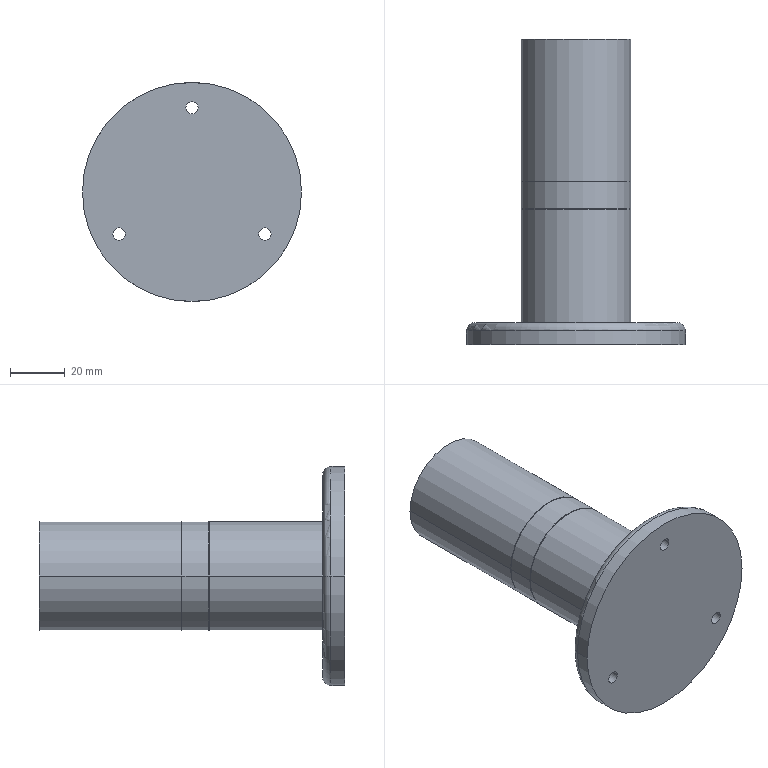Part | NX | 1 solid | 49 faces | box 80 x 111.49 x 80 mm | volume 113114 mm3 | cylinder 28 | plane 10 | torus 6 | cone 4 | sphere 1 | commonest cylinder face diameters 4.5 x6 6.5 x6 40 x6 10 x2 12 x2 36 x2
STEP:
#1=CARTESIAN_POINT('',(20.,-185.9,0.));
#2=VERTEX_POINT('',#1);
#3=CARTESIAN_POINT('',(-20.,-185.9,0.));
#4=VERTEX_POINT('',#3);
#5=CARTESIAN_POINT('',(0.,-185.9,0.));
#6=DIRECTION('',(0.,1.,0.));
#7=DIRECTION('',(1.,0.,0.));
#8=AXIS2_PLACEMENT_3D('',#5,#6,#7);
#9=CIRCLE('',#8,20.);
#10=EDGE_CURVE('',#2,#4,#9,.T.);
#11=ORIENTED_EDGE('',*,*,#10,.F.);
#12=CARTESIAN_POINT('',(19.9,-186.,0.));
#13=VERTEX_POINT('',#12);
#14=CARTESIAN_POINT('',(19.9,-185.9,0.));
#15=DIRECTION('',(0.,0.,1.));
#16=DIRECTION('',(1.,0.,0.));
#17=AXIS2_PLACEMENT_3D('',#14,#15,#16);
#18=CIRCLE('',#17,0.1);
#19=EDGE_CURVE('',#13,#2,#18,.T.);
#20=ORIENTED_EDGE('',*,*,#19,.F.);
#21=CARTESIAN_POINT('',(-19.9,-186.,0.));
#22=VERTEX_POINT('',#21);
#23=CARTESIAN_POINT('',(0.,-186.,0.));
#24=DIRECTION('',(0.,1.,0.));
#25=DIRECTION('',(-1.,0.,0.));
#26=AXIS2_PLACEMENT_3D('',#23,#24,#25);
#27=CIRCLE('',#26,19.9);
#28=EDGE_CURVE('',#13,#22,#27,.T.);
#29=ORIENTED_EDGE('',*,*,#28,.T.);
#30=CARTESIAN_POINT('',(-19.9,-185.9,0.));
#31=DIRECTION('',(0.,0.,-1.));
#32=DIRECTION('',(-1.,0.,0.));
#33=AXIS2_PLACEMENT_3D('',#30,#31,#32);
#34=CIRCLE('',#33,0.1);
#35=EDGE_CURVE('',#22,#4,#34,.T.);
#36=ORIENTED_EDGE('',*,*,#35,.T.);
#37=EDGE_LOOP('',(#11,#20,#29,#36));
#38=FACE_BOUND('',#37,.T.);
#39=CARTESIAN_POINT('',(0.,-185.9,0.));
#40=DIRECTION('',(0.,-1.,0.));
#41=DIRECTION('',(-1.,0.,0.));
#42=AXIS2_PLACEMENT_3D('',#39,#40,#41);
#43=TOROIDAL_SURFACE('',#42,19.9,0.1);
#44=ADVANCED_FACE('',(#38),#43,.T.);
#45=CARTESIAN_POINT('',(-40.,-230.5,0.));
#46=VERTEX_POINT('',#45);
#47=CARTESIAN_POINT('',(-37.,-227.5,0.));
#48=VERTEX_POINT('',#47);
#49=CARTESIAN_POINT('',(-37.,-230.5,0.));
#50=DIRECTION('',(0.,0.,-1.));
#51=DIRECTION('',(-1.,0.,0.));
#52=AXIS2_PLACEMENT_3D('',#49,#50,#51);
#53=CIRCLE('',#52,3.);
#54=EDGE_CURVE('',#46,#48,#53,.T.);
#55=ORIENTED_EDGE('',*,*,#54,.T.);
#56=CARTESIAN_POINT('',(37.,-227.5,0.));
#57=VERTEX_POINT('',#56);
#58=CARTESIAN_POINT('',(0.,-227.5,0.));
#59=DIRECTION('',(0.,-1.,0.));
#60=DIRECTION('',(1.,0.,0.));
#61=AXIS2_PLACEMENT_3D('',#58,#59,#60);
#62=CIRCLE('',#61,37.);
#63=EDGE_CURVE('',#48,#57,#62,.T.);
#64=ORIENTED_EDGE('',*,*,#63,.T.);
#65=CARTESIAN_POINT('',(40.,-230.5,0.));
#66=VERTEX_POINT('',#65);
#67=CARTESIAN_POINT('',(37.,-230.5,0.));
#68=DIRECTION('',(0.,0.,1.));
#69=DIRECTION('',(1.,0.,0.));
#70=AXIS2_PLACEMENT_3D('',#67,#68,#69);
#71=CIRCLE('',#70,3.);
#72=EDGE_CURVE('',#66,#57,#71,.T.);
#73=ORIENTED_EDGE('',*,*,#72,.F.);
#74=CARTESIAN_POINT('',(0.,-230.5,0.));
#75=DIRECTION('',(0.,-1.,0.));
#76=DIRECTION('',(-1.,0.,0.));
#77=AXIS2_PLACEMENT_3D('',#74,#75,#76);
#78=CIRCLE('',#77,40.);
#79=EDGE_CURVE('',#46,#66,#78,.T.);
#80=ORIENTED_EDGE('',*,*,#79,.F.);
#81=EDGE_LOOP('',(#55,#64,#73,#80));
#82=FACE_BOUND('',#81,.T.);
#83=CARTESIAN_POINT('',(0.,-230.5,0.));
#84=DIRECTION('',(0.,-1.,0.));
#85=DIRECTION('',(-1.,0.,0.));
#86=AXIS2_PLACEMENT_3D('',#83,#84,#85);
#87=TOROIDAL_SURFACE('',#86,37.,3.);
#88=ADVANCED_FACE('',(#82),#87,.T.);
#89=CARTESIAN_POINT('',(-20.,-186.1,0.));
#90=VERTEX_POINT('',#89);
#91=CARTESIAN_POINT('',(-19.9,-186.1,0.));
#92=DIRECTION('',(0.,0.,-1.));
#93=DIRECTION('',(-1.,0.,0.));
#94=AXIS2_PLACEMENT_3D('',#91,#92,#93);
#95=CIRCLE('',#94,0.1);
#96=EDGE_CURVE('',#90,#22,#95,.T.);
#97=ORIENTED_EDGE('',*,*,#96,.T.);
#98=ORIENTED_EDGE('',*,*,#28,.F.);
#99=CARTESIAN_POINT('',(20.,-186.1,0.));
#100=VERTEX_POINT('',#99);
#101=CARTESIAN_POINT('',(19.9,-186.1,0.));
#102=DIRECTION('',(0.,0.,1.));
#103=DIRECTION('',(1.,0.,0.));
#104=AXIS2_PLACEMENT_3D('',#101,#102,#103);
#105=CIRCLE('',#104,0.1);
#106=EDGE_CURVE('',#100,#13,#105,.T.);
#107=ORIENTED_EDGE('',*,*,#106,.F.);
#108=CARTESIAN_POINT('',(0.,-186.1,0.));
#109=DIRECTION('',(0.,-1.,0.));
#110=DIRECTION('',(-1.,0.,0.));
#111=AXIS2_PLACEMENT_3D('',#108,#109,#110);
#112=CIRCLE('',#111,20.);
#113=EDGE_CURVE('',#90,#100,#112,.T.);
#114=ORIENTED_EDGE('',*,*,#113,.F.);
#115=EDGE_LOOP('',(#97,#98,#107,#114));
#116=FACE_BOUND('',#115,.T.);
#117=CARTESIAN_POINT('',(0.,-186.1,0.));
#118=DIRECTION('',(0.,-1.,0.));
#119=DIRECTION('',(-1.,0.,0.));
#120=AXIS2_PLACEMENT_3D('',#117,#118,#119);
#121=TOROIDAL_SURFACE('',#120,19.9,0.1);
#122=ADVANCED_FACE('',(#116),#121,.T.);
#123=CARTESIAN_POINT('',(-18.,-175.95,0.));
#124=VERTEX_POINT('',#123);
#125=CARTESIAN_POINT('',(-18.,-124.01,0.));
#126=VERTEX_POINT('',#125);
#127=CARTESIAN_POINT('',(-18.,-120.91,0.));
#128=DIRECTION('',(0.,-1.,0.));
#129=VECTOR('',#128,1000.);
#130=LINE('',#127,#129);
#131=EDGE_CURVE('',#124,#126,#130,.F.);
#132=ORIENTED_EDGE('',*,*,#131,.T.);
#133=CARTESIAN_POINT('',(18.,-124.01,0.));
#134=VERTEX_POINT('',#133);
#135=CARTESIAN_POINT('',(0.,-124.01,0.));
#136=DIRECTION('',(0.,1.,0.));
#137=DIRECTION('',(1.,0.,0.));
#138=AXIS2_PLACEMENT_3D('',#135,#136,#137);
#139=CIRCLE('',#138,18.);
#140=EDGE_CURVE('',#126,#134,#139,.T.);
#141=ORIENTED_EDGE('',*,*,#140,.T.);
#142=CARTESIAN_POINT('',(18.,-175.95,0.));
#143=VERTEX_POINT('',#142);
#144=CARTESIAN_POINT('',(18.,-120.91,0.));
#145=DIRECTION('',(0.,-1.,0.));
#146=VECTOR('',#145,1000.);
#147=LINE('',#144,#146);
#148=EDGE_CURVE('',#143,#134,#147,.F.);
#149=ORIENTED_EDGE('',*,*,#148,.F.);
#150=CARTESIAN_POINT('',(0.,-175.95,0.));
#151=DIRECTION('',(0.,-1.,0.));
#152=DIRECTION('',(1.,0.,0.));
#153=AXIS2_PLACEMENT_3D('',#150,#151,#152);
#154=CIRCLE('',#153,18.);
#155=EDGE_CURVE('',#143,#124,#154,.T.);
#156=ORIENTED_EDGE('',*,*,#155,.T.);
#157=EDGE_LOOP('',(#132,#141,#149,#156));
#158=FACE_BOUND('',#157,.T.);
#159=CARTESIAN_POINT('',(0.,-120.91,0.));
#160=DIRECTION('',(0.,-1.,0.));
#161=DIRECTION('',(-1.,0.,0.));
#162=AXIS2_PLACEMENT_3D('',#159,#160,#161);
#163=CYLINDRICAL_SURFACE('',#162,18.);
#164=ADVANCED_FACE('',(#158),#163,.F.);
#165=CARTESIAN_POINT('',(-2.25,-229.5,30.75));
#166=VERTEX_POINT('',#165);
#167=CARTESIAN_POINT('',(2.25,-229.5,30.75));
#168=VERTEX_POINT('',#167);
#169=CARTESIAN_POINT('',(0.,-229.5,30.75));
#170=DIRECTION('',(0.,1.,0.));
#171=DIRECTION('',(1.,0.,0.));
#172=AXIS2_PLACEMENT_3D('',#169,#170,#171);
#173=CIRCLE('',#172,2.25);
#174=EDGE_CURVE('',#166,#168,#173,.T.);
#175=ORIENTED_EDGE('',*,*,#174,.T.);
#176=CARTESIAN_POINT('',(2.25,-235.5,30.75));
#177=VERTEX_POINT('',#176);
#178=CARTESIAN_POINT('',(2.25,-511.752,30.75));
#179=DIRECTION('',(0.,1.,0.));
#180=VECTOR('',#179,1000.);
#181=LINE('',#178,#180);
#182=EDGE_CURVE('',#177,#168,#181,.T.);
#183=ORIENTED_EDGE('',*,*,#182,.F.);
#184=CARTESIAN_POINT('',(-2.25,-235.5,30.75));
#185=VERTEX_POINT('',#184);
#186=CARTESIAN_POINT('',(0.,-235.5,30.75));
#187=DIRECTION('',(0.,-1.,0.));
#188=DIRECTION('',(1.,0.,0.));
#189=AXIS2_PLACEMENT_3D('',#186,#187,#188);
#190=CIRCLE('',#189,2.25);
#191=EDGE_CURVE('',#177,#185,#190,.T.);
#192=ORIENTED_EDGE('',*,*,#191,.T.);
#193=CARTESIAN_POINT('',(-2.25,-511.752,30.75));
#194=DIRECTION('',(0.,1.,0.));
#195=VECTOR('',#194,1000.);
#196=LINE('',#193,#195);
#197=EDGE_CURVE('',#185,#166,#196,.T.);
#198=ORIENTED_EDGE('',*,*,#197,.T.);
#199=EDGE_LOOP('',(#175,#183,#192,#198));
#200=FACE_BOUND('',#199,.T.);
#201=CARTESIAN_POINT('',(0.,-511.752,30.75));
#202=DIRECTION('',(0.,1.,0.));
#203=DIRECTION('',(1.,0.,0.));
#204=AXIS2_PLACEMENT_3D('',#201,#202,#203);
#205=CYLINDRICAL_SURFACE('',#204,2.25);
#206=ADVANCED_FACE('',(#200),#205,.F.);
#207=CARTESIAN_POINT('',(29.88,-227.5,-15.375));
#208=VERTEX_POINT('',#207);
#209=CARTESIAN_POINT('',(29.88,-229.5,-15.375));
#210=VERTEX_POINT('',#209);
#211=CARTESIAN_POINT('',(29.88,-503.23,-15.375));
#212=DIRECTION('',(0.,1.,0.));
#213=VECTOR('',#212,1000.);
#214=LINE('',#211,#213);
#215=EDGE_CURVE('',#208,#210,#214,.F.);
#216=ORIENTED_EDGE('',*,*,#215,.F.);
#217=CARTESIAN_POINT('',(23.38,-227.5,-15.375));
#218=VERTEX_POINT('',#217);
#219=CARTESIAN_POINT('',(26.63,-227.5,-15.375));
#220=DIRECTION('',(0.,1.,0.));
#221=DIRECTION('',(-1.,0.,0.));
#222=AXIS2_PLACEMENT_3D('',#219,#220,#221);
#223=CIRCLE('',#222,3.25);
#224=EDGE_CURVE('',#208,#218,#223,.T.);
#225=ORIENTED_EDGE('',*,*,#224,.T.);
#226=CARTESIAN_POINT('',(23.38,-229.5,-15.375));
#227=VERTEX_POINT('',#226);
#228=CARTESIAN_POINT('',(23.38,-503.23,-15.375));
#229=DIRECTION('',(0.,1.,0.));
#230=VECTOR('',#229,1000.);
#231=LINE('',#228,#230);
#232=EDGE_CURVE('',#218,#227,#231,.F.);
#233=ORIENTED_EDGE('',*,*,#232,.T.);
#234=CARTESIAN_POINT('',(26.63,-229.5,-15.375));
#235=DIRECTION('',(0.,-1.,0.));
#236=DIRECTION('',(1.,0.,0.));
#237=AXIS2_PLACEMENT_3D('',#234,#235,#236);
#238=CIRCLE('',#237,3.25);
#239=EDGE_CURVE('',#227,#210,#238,.T.);
#240=ORIENTED_EDGE('',*,*,#239,.T.);
#241=EDGE_LOOP('',(#216,#225,#233,#240));
#242=FACE_BOUND('',#241,.T.);
#243=CARTESIAN_POINT('',(26.63,-503.23,-15.375));
#244=DIRECTION('',(0.,1.,0.));
#245=DIRECTION('',(1.,0.,0.));
#246=AXIS2_PLACEMENT_3D('',#243,#244,#245);
#247=CYLINDRICAL_SURFACE('',#246,3.25);
#248=ADVANCED_FACE('',(#242),#247,.F.);
#249=CARTESIAN_POINT('',(-23.38,-227.5,-15.375));
#250=VERTEX_POINT('',#249);
#251=CARTESIAN_POINT('',(-23.38,-229.5,-15.375));
#252=VERTEX_POINT('',#251);
#253=CARTESIAN_POINT('',(-23.38,-503.23,-15.375));
#254=DIRECTION('',(0.,1.,0.));
#255=VECTOR('',#254,1000.);
#256=LINE('',#253,#255);
#257=EDGE_CURVE('',#250,#252,#256,.F.);
#258=ORIENTED_EDGE('',*,*,#257,.F.);
#259=CARTESIAN_POINT('',(-29.88,-227.5,-15.375));
#260=VERTEX_POINT('',#259);
#261=CARTESIAN_POINT('',(-26.63,-227.5,-15.375));
#262=DIRECTION('',(0.,1.,0.));
#263=DIRECTION('',(-1.,0.,0.));
#264=AXIS2_PLACEMENT_3D('',#261,#262,#263);
#265=CIRCLE('',#264,3.25);
#266=EDGE_CURVE('',#250,#260,#265,.T.);
#267=ORIENTED_EDGE('',*,*,#266,.T.);
#268=CARTESIAN_POINT('',(-29.88,-229.5,-15.375));
#269=VERTEX_POINT('',#268);
#270=CARTESIAN_POINT('',(-29.88,-503.23,-15.375));
#271=DIRECTION('',(0.,1.,0.));
#272=VECTOR('',#271,1000.);
#273=LINE('',#270,#272);
#274=EDGE_CURVE('',#260,#269,#273,.F.);
#275=ORIENTED_EDGE('',*,*,#274,.T.);
#276=CARTESIAN_POINT('',(-26.63,-229.5,-15.375));
#277=DIRECTION('',(0.,-1.,0.));
#278=DIRECTION('',(1.,0.,0.));
#279=AXIS2_PLACEMENT_3D('',#276,#277,#278);
#280=CIRCLE('',#279,3.25);
#281=EDGE_CURVE('',#269,#252,#280,.T.);
#282=ORIENTED_EDGE('',*,*,#281,.T.);
#283=EDGE_LOOP('',(#258,#267,#275,#282));
#284=FACE_BOUND('',#283,.T.);
#285=CARTESIAN_POINT('',(-26.63,-503.23,-15.375));
#286=DIRECTION('',(0.,1.,0.));
#287=DIRECTION('',(1.,0.,0.));
#288=AXIS2_PLACEMENT_3D('',#285,#286,#287);
#289=CYLINDRICAL_SURFACE('',#288,3.25);
#290=ADVANCED_FACE('',(#284),#289,.F.);
#291=CARTESIAN_POINT('',(-20.,-176.05,0.));
#292=VERTEX_POINT('',#291);
#293=CARTESIAN_POINT('',(-19.95,-176.,0.));
#294=VERTEX_POINT('',#293);
#295=CARTESIAN_POINT('',(-19.975,-176.025,0.));
#296=DIRECTION('',(-0.7071,-0.7071,0.));
#297=VECTOR('',#296,1000.);
#298=LINE('',#295,#297);
#299=EDGE_CURVE('',#292,#294,#298,.F.);
#300=ORIENTED_EDGE('',*,*,#299,.F.);
#301=CARTESIAN_POINT('',(20.,-176.05,0.));
#302=VERTEX_POINT('',#301);
#303=CARTESIAN_POINT('',(0.,-176.05,0.));
#304=DIRECTION('',(0.,-1.,0.));
#305=DIRECTION('',(1.,0.,0.));
#306=AXIS2_PLACEMENT_3D('',#303,#304,#305);
#307=CIRCLE('',#306,20.);
#308=EDGE_CURVE('',#302,#292,#307,.T.);
#309=ORIENTED_EDGE('',*,*,#308,.F.);
#310=CARTESIAN_POINT('',(19.95,-176.,0.));
#311=VERTEX_POINT('',#310);
#312=CARTESIAN_POINT('',(19.975,-176.025,0.));
#313=DIRECTION('',(0.7071,-0.7071,0.));
#314=VECTOR('',#313,1000.);
#315=LINE('',#312,#314);
#316=EDGE_CURVE('',#302,#311,#315,.F.);
#317=ORIENTED_EDGE('',*,*,#316,.T.);
#318=CARTESIAN_POINT('',(0.,-176.,0.));
#319=DIRECTION('',(0.,1.,0.));
#320=DIRECTION('',(-1.,0.,0.));
#321=AXIS2_PLACEMENT_3D('',#318,#319,#320);
#322=CIRCLE('',#321,19.95);
#323=EDGE_CURVE('',#294,#311,#322,.T.);
#324=ORIENTED_EDGE('',*,*,#323,.F.);
#325=EDGE_LOOP('',(#300,#309,#317,#324));
#326=FACE_BOUND('',#325,.T.);
#327=CARTESIAN_POINT('',(0.,-176.025,0.));
#328=DIRECTION('',(0.,-1.,0.));
#329=DIRECTION('',(-1.,0.,0.));
#330=AXIS2_PLACEMENT_3D('',#327,#328,#329);
#331=CONICAL_SURFACE('',#330,19.975,0.7854);
#332=ADVANCED_FACE('',(#326),#331,.T.);
#333=CARTESIAN_POINT('',(-19.85,-175.95,0.));
#334=VERTEX_POINT('',#333);
#335=CARTESIAN_POINT('',(-19.85,-176.,0.));
#336=VERTEX_POINT('',#335);
#337=CARTESIAN_POINT('',(-19.85,-120.91,0.));
#338=DIRECTION('',(0.,-1.,0.));
#339=VECTOR('',#338,1000.);
#340=LINE('',#337,#339);
#341=EDGE_CURVE('',#334,#336,#340,.T.);
#342=ORIENTED_EDGE('',*,*,#341,.F.);
#343=CARTESIAN_POINT('',(19.85,-175.95,0.));
#344=VERTEX_POINT('',#343);
#345=CARTESIAN_POINT('',(0.,-175.95,0.));
#346=DIRECTION('',(0.,1.,0.));
#347=DIRECTION('',(1.,0.,0.));
#348=AXIS2_PLACEMENT_3D('',#345,#346,#347);
#349=CIRCLE('',#348,19.85);
#350=EDGE_CURVE('',#334,#344,#349,.T.);
#351=ORIENTED_EDGE('',*,*,#350,.T.);
#352=CARTESIAN_POINT('',(19.85,-176.,0.));
#353=VERTEX_POINT('',#352);
#354=CARTESIAN_POINT('',(19.85,-120.91,0.));
#355=DIRECTION('',(0.,-1.,0.));
#356=VECTOR('',#355,1000.);
#357=LINE('',#354,#356);
#358=EDGE_CURVE('',#344,#353,#357,.T.);
#359=ORIENTED_EDGE('',*,*,#358,.T.);
#360=CARTESIAN_POINT('',(0.,-176.,0.));
#361=DIRECTION('',(0.,-1.,0.));
#362=DIRECTION('',(1.,0.,0.));
#363=AXIS2_PLACEMENT_3D('',#360,#361,#362);
#364=CIRCLE('',#363,19.85);
#365=EDGE_CURVE('',#353,#336,#364,.T.);
#366=ORIENTED_EDGE('',*,*,#365,.T.);
#367=EDGE_LOOP('',(#342,#351,#359,#366));
#368=FACE_BOUND('',#367,.T.);
#369=CARTESIAN_POINT('',(0.,-120.91,0.));
#370=DIRECTION('',(0.,-1.,0.));
#371=DIRECTION('',(-1.,0.,0.));
#372=AXIS2_PLACEMENT_3D('',#369,#370,#371);
#373=CYLINDRICAL_SURFACE('',#372,19.85);
#374=ADVANCED_FACE('',(#368),#373,.F.);
#375=CARTESIAN_POINT('',(-40.,-235.5,0.));
#376=VERTEX_POINT('',#375);
#377=CARTESIAN_POINT('',(-40.,-227.1,0.));
#378=DIRECTION('',(0.,-1.,0.));
#379=VECTOR('',#378,1000.);
#380=LINE('',#377,#379);
#381=EDGE_CURVE('',#376,#46,#380,.F.);
#382=ORIENTED_EDGE('',*,*,#381,.T.);
#383=ORIENTED_EDGE('',*,*,#79,.T.);
#384=CARTESIAN_POINT('',(40.,-235.5,0.));
#385=VERTEX_POINT('',#384);
#386=CARTESIAN_POINT('',(40.,-227.1,0.));
#387=DIRECTION('',(0.,-1.,0.));
#388=VECTOR('',#387,1000.);
#389=LINE('',#386,#388);
#390=EDGE_CURVE('',#385,#66,#389,.F.);
#391=ORIENTED_EDGE('',*,*,#390,.F.);
#392=CARTESIAN_POINT('',(0.,-235.5,0.));
#393=DIRECTION('',(0.,1.,0.));
#394=DIRECTION('',(1.,0.,0.));
#395=AXIS2_PLACEMENT_3D('',#392,#393,#394);
#396=CIRCLE('',#395,40.);
#397=EDGE_CURVE('',#385,#376,#396,.T.);
#398=ORIENTED_EDGE('',*,*,#397,.T.);
#399=EDGE_LOOP('',(#382,#383,#391,#398));
#400=FACE_BOUND('',#399,.T.);
#401=CARTESIAN_POINT('',(0.,-227.1,0.));
#402=DIRECTION('',(0.,-1.,0.));
#403=DIRECTION('',(-1.,0.,0.));
#404=AXIS2_PLACEMENT_3D('',#401,#402,#403);
#405=CYLINDRICAL_SURFACE('',#404,40.);
#406=ADVANCED_FACE('',(#400),#405,.T.);
#407=CARTESIAN_POINT('',(24.38,-229.5,-15.375));
#408=VERTEX_POINT('',#407);
#409=CARTESIAN_POINT('',(28.88,-229.5,-15.375));
#410=VERTEX_POINT('',#409);
#411=CARTESIAN_POINT('',(26.63,-229.5,-15.375));
#412=DIRECTION('',(0.,1.,0.));
#413=DIRECTION('',(1.,0.,0.));
#414=AXIS2_PLACEMENT_3D('',#411,#412,#413);
#415=CIRCLE('',#414,2.25);
#416=EDGE_CURVE('',#408,#410,#415,.T.);
#417=ORIENTED_EDGE('',*,*,#416,.T.);
#418=CARTESIAN_POINT('',(28.88,-235.5,-15.375));
#419=VERTEX_POINT('',#418);
#420=CARTESIAN_POINT('',(28.88,-503.23,-15.375));
#421=DIRECTION('',(0.,1.,0.));
#422=VECTOR('',#421,1000.);
#423=LINE('',#420,#422);
#424=EDGE_CURVE('',#419,#410,#423,.T.);
#425=ORIENTED_EDGE('',*,*,#424,.F.);
#426=CARTESIAN_POINT('',(24.38,-235.5,-15.375));
#427=VERTEX_POINT('',#426);
#428=CARTESIAN_POINT('',(26.63,-235.5,-15.375));
#429=DIRECTION('',(0.,-1.,0.));
#430=DIRECTION('',(1.,0.,0.));
#431=AXIS2_PLACEMENT_3D('',#428,#429,#430);
#432=CIRCLE('',#431,2.25);
#433=EDGE_CURVE('',#419,#427,#432,.T.);
#434=ORIENTED_EDGE('',*,*,#433,.T.);
#435=CARTESIAN_POINT('',(24.38,-503.23,-15.375));
#436=DIRECTION('',(0.,1.,0.));
#437=VECTOR('',#436,1000.);
#438=LINE('',#435,#437);
#439=EDGE_CURVE('',#427,#408,#438,.T.);
#440=ORIENTED_EDGE('',*,*,#439,.T.);
#441=EDGE_LOOP('',(#417,#425,#434,#440));
#442=FACE_BOUND('',#441,.T.);
#443=CARTESIAN_POINT('',(26.63,-503.23,-15.375));
#444=DIRECTION('',(0.,1.,0.));
#445=DIRECTION('',(1.,0.,0.));
#446=AXIS2_PLACEMENT_3D('',#443,#444,#445);
#447=CYLINDRICAL_SURFACE('',#446,2.25);
#448=ADVANCED_FACE('',(#442),#447,.F.);
#449=CARTESIAN_POINT('',(-24.38,-235.5,-15.375));
#450=VERTEX_POINT('',#449);
#451=CARTESIAN_POINT('',(-24.38,-229.5,-15.375));
#452=VERTEX_POINT('',#451);
#453=CARTESIAN_POINT('',(-24.38,-503.23,-15.375));
#454=DIRECTION('',(0.,1.,0.));
#455=VECTOR('',#454,1000.);
#456=LINE('',#453,#455);
#457=EDGE_CURVE('',#450,#452,#456,.T.);
#458=ORIENTED_EDGE('',*,*,#457,.F.);
#459=CARTESIAN_POINT('',(-28.88,-235.5,-15.375));
#460=VERTEX_POINT('',#459);
#461=CARTESIAN_POINT('',(-26.63,-235.5,-15.375));
#462=DIRECTION('',(0.,-1.,0.));
#463=DIRECTION('',(1.,0.,0.));
#464=AXIS2_PLACEMENT_3D('',#461,#462,#463);
#465=CIRCLE('',#464,2.25);
#466=EDGE_CURVE('',#450,#460,#465,.T.);
#467=ORIENTED_EDGE('',*,*,#466,.T.);
#468=CARTESIAN_POINT('',(-28.88,-229.5,-15.375));
#469=VERTEX_POINT('',#468);
#470=CARTESIAN_POINT('',(-28.88,-503.23,-15.375));
#471=DIRECTION('',(0.,1.,0.));
#472=VECTOR('',#471,1000.);
#473=LINE('',#470,#472);
#474=EDGE_CURVE('',#460,#469,#473,.T.);
#475=ORIENTED_EDGE('',*,*,#474,.T.);
#476=CARTESIAN_POINT('',(-26.63,-229.5,-15.375));
#477=DIRECTION('',(0.,1.,0.));
#478=DIRECTION('',(-1.,0.,0.));
#479=AXIS2_PLACEMENT_3D('',#476,#477,#478);
#480=CIRCLE('',#479,2.25);
#481=EDGE_CURVE('',#469,#452,#480,.T.);
#482=ORIENTED_EDGE('',*,*,#481,.T.);
#483=EDGE_LOOP('',(#458,#467,#475,#482));
#484=FACE_BOUND('',#483,.T.);
#485=CARTESIAN_POINT('',(-26.63,-503.23,-15.375));
#486=DIRECTION('',(0.,1.,0.));
#487=DIRECTION('',(1.,0.,0.));
#488=AXIS2_PLACEMENT_3D('',#485,#486,#487);
#489=CYLINDRICAL_SURFACE('',#488,2.25);
#490=ADVANCED_FACE('',(#484),#489,.F.);
#491=CARTESIAN_POINT('',(-20.,-227.5,0.));
#492=VERTEX_POINT('',#491);
#493=CARTESIAN_POINT('',(-20.,-183.925,0.));
#494=DIRECTION('',(0.,-1.,0.));
#495=VECTOR('',#494,1000.);
#496=LINE('',#493,#495);
#497=EDGE_CURVE('',#492,#90,#496,.F.);
#498=ORIENTED_EDGE('',*,*,#497,.T.);
#499=ORIENTED_EDGE('',*,*,#113,.T.);
#500=CARTESIAN_POINT('',(20.,-227.5,0.));
#501=VERTEX_POINT('',#500);
#502=CARTESIAN_POINT('',(20.,-183.925,0.));
#503=DIRECTION('',(0.,-1.,0.));
#504=VECTOR('',#503,1000.);
#505=LINE('',#502,#504);
#506=EDGE_CURVE('',#501,#100,#505,.F.);
#507=ORIENTED_EDGE('',*,*,#506,.F.);
#508=CARTESIAN_POINT('',(0.,-227.5,0.));
#509=DIRECTION('',(0.,1.,0.));
#510=DIRECTION('',(1.,0.,0.));
#511=AXIS2_PLACEMENT_3D('',#508,#509,#510);
#512=CIRCLE('',#511,20.);
#513=EDGE_CURVE('',#501,#492,#512,.T.);
#514=ORIENTED_EDGE('',*,*,#513,.T.);
#515=EDGE_LOOP('',(#498,#499,#507,#514));
#516=FACE_BOUND('',#515,.T.);
#517=CARTESIAN_POINT('',(0.,-183.925,0.));
#518=DIRECTION('',(0.,-1.,0.));
#519=DIRECTION('',(-1.,0.,0.));
#520=AXIS2_PLACEMENT_3D('',#517,#518,#519);
#521=CYLINDRICAL_SURFACE('',#520,20.);
#522=ADVANCED_FACE('',(#516),#521,.T.);
#523=CARTESIAN_POINT('',(-20.,-120.91,0.));
#524=DIRECTION('',(0.,-1.,0.));
#525=VECTOR('',#524,1000.);
#526=LINE('',#523,#525);
#527=EDGE_CURVE('',#4,#292,#526,.F.);
#528=ORIENTED_EDGE('',*,*,#527,.F.);
#529=CARTESIAN_POINT('',(0.,-185.9,0.));
#530=DIRECTION('',(0.,1.,0.));
#531=DIRECTION('',(1.,0.,0.));
#532=AXIS2_PLACEMENT_3D('',#529,#530,#531);
#533=CIRCLE('',#532,20.);
#534=EDGE_CURVE('',#4,#2,#533,.T.);
#535=ORIENTED_EDGE('',*,*,#534,.T.);
#536=CARTESIAN_POINT('',(20.,-120.91,0.));
#537=DIRECTION('',(0.,-1.,0.));
#538=VECTOR('',#537,1000.);
#539=LINE('',#536,#538);
#540=EDGE_CURVE('',#2,#302,#539,.F.);
#541=ORIENTED_EDGE('',*,*,#540,.T.);
#542=ORIENTED_EDGE('',*,*,#308,.T.);
#543=EDGE_LOOP('',(#528,#535,#541,#542));
#544=FACE_BOUND('',#543,.T.);
#545=CARTESIAN_POINT('',(0.,-120.91,0.));
#546=DIRECTION('',(0.,-1.,0.));
#547=DIRECTION('',(-1.,0.,0.));
#548=AXIS2_PLACEMENT_3D('',#545,#546,#547);
#549=CYLINDRICAL_SURFACE('',#548,20.);
#550=ADVANCED_FACE('',(#544),#549,.T.);
#551=CARTESIAN_POINT('',(-20.,-175.95,0.));
#552=VERTEX_POINT('',#551);
#553=CARTESIAN_POINT('',(-20.,-124.01,0.));
#554=VERTEX_POINT('',#553);
#555=CARTESIAN_POINT('',(-20.,-120.91,0.));
#556=DIRECTION('',(0.,-1.,0.));
#557=VECTOR('',#556,1000.);
#558=LINE('',#555,#557);
#559=EDGE_CURVE('',#552,#554,#558,.F.);
#560=ORIENTED_EDGE('',*,*,#559,.F.);
#561=CARTESIAN_POINT('',(20.,-175.95,0.));
#562=VERTEX_POINT('',#561);
#563=CARTESIAN_POINT('',(0.,-175.95,0.));
#564=DIRECTION('',(0.,1.,0.));
#565=DIRECTION('',(1.,0.,0.));
#566=AXIS2_PLACEMENT_3D('',#563,#564,#565);
#567=CIRCLE('',#566,20.);
#568=EDGE_CURVE('',#552,#562,#567,.T.);
#569=ORIENTED_EDGE('',*,*,#568,.T.);
#570=CARTESIAN_POINT('',(20.,-124.01,0.));
#571=VERTEX_POINT('',#570);
#572=CARTESIAN_POINT('',(20.,-120.91,0.));
#573=DIRECTION('',(0.,-1.,0.));
#574=VECTOR('',#573,1000.);
#575=LINE('',#572,#574);
#576=EDGE_CURVE('',#562,#571,#575,.F.);
#577=ORIENTED_EDGE('',*,*,#576,.T.);
#578=CARTESIAN_POINT('',(0.,-124.01,0.));
#579=DIRECTION('',(0.,-1.,0.));
#580=DIRECTION('',(1.,0.,0.));
#581=AXIS2_PLACEMENT_3D('',#578,#579,#580);
#582=CIRCLE('',#581,20.);
#583=EDGE_CURVE('',#571,#554,#582,.T.);
#584=ORIENTED_EDGE('',*,*,#583,.T.);
#585=EDGE_LOOP('',(#560,#569,#577,#584));
#586=FACE_BOUND('',#585,.T.);
#587=CARTESIAN_POINT('',(0.,-120.91,0.));
#588=DIRECTION('',(0.,-1.,0.));
#589=DIRECTION('',(-1.,0.,0.));
#590=AXIS2_PLACEMENT_3D('',#587,#588,#589);
#591=CYLINDRICAL_SURFACE('',#590,20.);
#592=ADVANCED_FACE('',(#586),#591,.T.);
#593=CARTESIAN_POINT('',(-3.25,-227.5,30.75));
#594=VERTEX_POINT('',#593);
#595=CARTESIAN_POINT('',(3.25,-227.5,30.75));
#596=VERTEX_POINT('',#595);
#597=CARTESIAN_POINT('',(0.,-227.5,30.75));
#598=DIRECTION('',(0.,1.,0.));
#599=DIRECTION('',(1.,0.,0.));
#600=AXIS2_PLACEMENT_3D('',#597,#598,#599);
#601=CIRCLE('',#600,3.25);
#602=EDGE_CURVE('',#594,#596,#601,.T.);
#603=ORIENTED_EDGE('',*,*,#602,.T.);
#604=CARTESIAN_POINT('',(3.25,-229.5,30.75));
#605=VERTEX_POINT('',#604);
#606=CARTESIAN_POINT('',(3.25,-511.752,30.75));
#607=DIRECTION('',(0.,1.,0.));
#608=VECTOR('',#607,1000.);
#609=LINE('',#606,#608);
#610=EDGE_CURVE('',#605,#596,#609,.T.);
#611=ORIENTED_EDGE('',*,*,#610,.F.);
#612=CARTESIAN_POINT('',(-3.25,-229.5,30.75));
#613=VERTEX_POINT('',#612);
#614=CARTESIAN_POINT('',(0.,-229.5,30.75));
#615=DIRECTION('',(0.,-1.,0.));
#616=DIRECTION('',(1.,0.,0.));
#617=AXIS2_PLACEMENT_3D('',#614,#615,#616);
#618=CIRCLE('',#617,3.25);
#619=EDGE_CURVE('',#605,#613,#618,.T.);
#620=ORIENTED_EDGE('',*,*,#619,.T.);
#621=CARTESIAN_POINT('',(-3.25,-511.752,30.75));
#622=DIRECTION('',(0.,1.,0.));
#623=VECTOR('',#622,1000.);
#624=LINE('',#621,#623);
#625=EDGE_CURVE('',#613,#594,#624,.T.);
#626=ORIENTED_EDGE('',*,*,#625,.T.);
#627=EDGE_LOOP('',(#603,#611,#620,#626));
#628=FACE_BOUND('',#627,.T.);
#629=CARTESIAN_POINT('',(0.,-511.752,30.75));
#630=DIRECTION('',(0.,1.,0.));
#631=DIRECTION('',(1.,0.,0.));
#632=AXIS2_PLACEMENT_3D('',#629,#630,#631);
#633=CYLINDRICAL_SURFACE('',#632,3.25);
#634=ADVANCED_FACE('',(#628),#633,.F.);
#635=CARTESIAN_POINT('',(-5.,-176.,0.));
#636=VERTEX_POINT('',#635);
#637=CARTESIAN_POINT('',(-5.,-161.,0.));
#638=VERTEX_POINT('',#637);
#639=CARTESIAN_POINT('',(-5.,-120.91,0.));
#640=DIRECTION('',(0.,-1.,0.));
#641=VECTOR('',#640,1000.);
#642=LINE('',#639,#641);
#643=EDGE_CURVE('',#636,#638,#642,.F.);
#644=ORIENTED_EDGE('',*,*,#643,.F.);
#645=CARTESIAN_POINT('',(5.,-176.,0.));
#646=VERTEX_POINT('',#645);
#647=CARTESIAN_POINT('',(0.,-176.,0.));
#648=DIRECTION('',(0.,1.,0.));
#649=DIRECTION('',(1.,0.,0.));
#650=AXIS2_PLACEMENT_3D('',#647,#648,#649);
#651=CIRCLE('',#650,5.);
#652=EDGE_CURVE('',#636,#646,#651,.T.);
#653=ORIENTED_EDGE('',*,*,#652,.T.);
#654=CARTESIAN_POINT('',(5.,-161.,0.));
#655=VERTEX_POINT('',#654);
#656=CARTESIAN_POINT('',(5.,-120.91,0.));
#657=DIRECTION('',(0.,-1.,0.));
#658=VECTOR('',#657,1000.);
#659=LINE('',#656,#658);
#660=EDGE_CURVE('',#646,#655,#659,.F.);
#661=ORIENTED_EDGE('',*,*,#660,.T.);
#662=CARTESIAN_POINT('',(0.,-161.,0.));
#663=DIRECTION('',(0.,1.,0.));
#664=DIRECTION('',(1.,0.,0.));
#665=AXIS2_PLACEMENT_3D('',#662,#663,#664);
#666=CIRCLE('',#665,5.);
#667=EDGE_CURVE('',#638,#655,#666,.T.);
#668=ORIENTED_EDGE('',*,*,#667,.F.);
#669=EDGE_LOOP('',(#644,#653,#661,#668));
#670=FACE_BOUND('',#669,.T.);
#671=CARTESIAN_POINT('',(0.,-120.91,0.));
#672=DIRECTION('',(0.,-1.,0.));
#673=DIRECTION('',(-1.,0.,0.));
#674=AXIS2_PLACEMENT_3D('',#671,#672,#673);
#675=CYLINDRICAL_SURFACE('',#674,5.);
#676=ADVANCED_FACE('',(#670),#675,.T.);
#677=CARTESIAN_POINT('',(19.975,-175.975,0.));
#678=DIRECTION('',(0.7071,0.7071,0.));
#679=VECTOR('',#678,1000.);
#680=LINE('',#677,#679);
#681=EDGE_CURVE('',#311,#562,#680,.T.);
#682=ORIENTED_EDGE('',*,*,#681,.T.);
#683=ORIENTED_EDGE('',*,*,#568,.F.);
#684=CARTESIAN_POINT('',(-19.975,-175.975,0.));
#685=DIRECTION('',(-0.7071,0.7071,0.));
#686=VECTOR('',#685,1000.);
#687=LINE('',#684,#686);
#688=EDGE_CURVE('',#294,#552,#687,.T.);
#689=ORIENTED_EDGE('',*,*,#688,.F.);
#690=ORIENTED_EDGE('',*,*,#323,.T.);
#691=EDGE_LOOP('',(#682,#683,#689,#690));
#692=FACE_BOUND('',#691,.T.);
#693=CARTESIAN_POINT('',(0.,-175.975,0.));
#694=DIRECTION('',(0.,1.,0.));
#695=DIRECTION('',(1.,0.,0.));
#696=AXIS2_PLACEMENT_3D('',#693,#694,#695);
#697=CONICAL_SURFACE('',#696,19.975,0.7854);
#698=ADVANCED_FACE('',(#692),#697,.T.);
#699=CARTESIAN_POINT('',(0.,-176.,0.));
#700=DIRECTION('',(0.,-1.,0.));
#701=DIRECTION('',(1.,0.,0.));
#702=AXIS2_PLACEMENT_3D('',#699,#700,#701);
#703=CIRCLE('',#702,19.85);
#704=EDGE_CURVE('',#336,#353,#703,.T.);
#705=ORIENTED_EDGE('',*,*,#704,.T.);
#706=ORIENTED_EDGE('',*,*,#358,.F.);
#707=CARTESIAN_POINT('',(0.,-175.95,0.));
#708=DIRECTION('',(0.,1.,0.));
#709=DIRECTION('',(1.,0.,0.));
#710=AXIS2_PLACEMENT_3D('',#707,#708,#709);
#711=CIRCLE('',#710,19.85);
#712=EDGE_CURVE('',#344,#334,#711,.T.);
#713=ORIENTED_EDGE('',*,*,#712,.T.);
#714=ORIENTED_EDGE('',*,*,#341,.T.);
#715=EDGE_LOOP('',(#705,#706,#713,#714));
#716=FACE_BOUND('',#715,.T.);
#717=CARTESIAN_POINT('',(0.,-120.91,0.));
#718=DIRECTION('',(0.,-1.,0.));
#719=DIRECTION('',(-1.,0.,0.));
#720=AXIS2_PLACEMENT_3D('',#717,#718,#719);
#721=CYLINDRICAL_SURFACE('',#720,19.85);
#722=ADVANCED_FACE('',(#716),#721,.F.);
#723=CARTESIAN_POINT('',(0.,-186.,0.));
#724=DIRECTION('',(0.,1.,0.));
#725=DIRECTION('',(-1.,0.,0.));
#726=AXIS2_PLACEMENT_3D('',#723,#724,#725);
#727=CIRCLE('',#726,19.9);
#728=EDGE_CURVE('',#22,#13,#727,.T.);
#729=ORIENTED_EDGE('',*,*,#728,.T.);
#730=ORIENTED_EDGE('',*,*,#19,.T.);
#731=ORIENTED_EDGE('',*,*,#534,.F.);
#732=ORIENTED_EDGE('',*,*,#35,.F.);
#733=EDGE_LOOP('',(#729,#730,#731,#732));
#734=FACE_BOUND('',#733,.T.);
#735=CARTESIAN_POINT('',(0.,-185.9,0.));
#736=DIRECTION('',(0.,-1.,0.));
#737=DIRECTION('',(-1.,0.,0.));
#738=AXIS2_PLACEMENT_3D('',#735,#736,#737);
#739=TOROIDAL_SURFACE('',#738,19.9,0.1);
#740=ADVANCED_FACE('',(#734),#739,.T.);
#741=CARTESIAN_POINT('',(0.,-124.01,0.));
#742=DIRECTION('',(0.,1.,0.));
#743=DIRECTION('',(1.,0.,0.));
#744=AXIS2_PLACEMENT_3D('',#741,#742,#743);
#745=CIRCLE('',#744,18.);
#746=EDGE_CURVE('',#134,#126,#745,.T.);
#747=ORIENTED_EDGE('',*,*,#746,.F.);
#748=ORIENTED_EDGE('',*,*,#140,.F.);
#749=EDGE_LOOP('',(#747,#748));
#750=FACE_BOUND('',#749,.T.);
#751=CARTESIAN_POINT('',(0.,-124.01,0.));
#752=DIRECTION('',(0.,-1.,0.));
#753=DIRECTION('',(1.,0.,0.));
#754=AXIS2_PLACEMENT_3D('',#751,#752,#753);
#755=CIRCLE('',#754,20.);
#756=EDGE_CURVE('',#554,#571,#755,.T.);
#757=ORIENTED_EDGE('',*,*,#756,.F.);
#758=ORIENTED_EDGE('',*,*,#583,.F.);
#759=EDGE_LOOP('',(#757,#758));
#760=FACE_BOUND('',#759,.T.);
#761=CARTESIAN_POINT('',(0.,-124.01,0.));
#762=DIRECTION('',(0.,-1.,0.));
#763=DIRECTION('',(0.,0.,-1.));
#764=AXIS2_PLACEMENT_3D('',#761,#762,#763);
#765=PLANE('',#764);
#766=ADVANCED_FACE('',(#750,#760),#765,.F.);
#767=CARTESIAN_POINT('',(0.,-186.1,0.));
#768=DIRECTION('',(0.,-1.,0.));
#769=DIRECTION('',(-1.,0.,0.));
#770=AXIS2_PLACEMENT_3D('',#767,#768,#769);
#771=CIRCLE('',#770,20.);
#772=EDGE_CURVE('',#100,#90,#771,.T.);
#773=ORIENTED_EDGE('',*,*,#772,.F.);
#774=ORIENTED_EDGE('',*,*,#106,.T.);
#775=ORIENTED_EDGE('',*,*,#728,.F.);
#776=ORIENTED_EDGE('',*,*,#96,.F.);
#777=EDGE_LOOP('',(#773,#774,#775,#776));
#778=FACE_BOUND('',#777,.T.);
#779=CARTESIAN_POINT('',(0.,-186.1,0.));
#780=DIRECTION('',(0.,-1.,0.));
#781=DIRECTION('',(-1.,0.,0.));
#782=AXIS2_PLACEMENT_3D('',#779,#780,#781);
#783=TOROIDAL_SURFACE('',#782,19.9,0.1);
#784=ADVANCED_FACE('',(#778),#783,.T.);
#785=ORIENTED_EDGE('',*,*,#643,.T.);
#786=CARTESIAN_POINT('',(0.,-161.,0.));
#787=DIRECTION('',(0.,1.,0.));
#788=DIRECTION('',(1.,0.,0.));
#789=AXIS2_PLACEMENT_3D('',#786,#787,#788);
#790=CIRCLE('',#789,5.);
#791=EDGE_CURVE('',#655,#638,#790,.T.);
#792=ORIENTED_EDGE('',*,*,#791,.F.);
#793=ORIENTED_EDGE('',*,*,#660,.F.);
#794=CARTESIAN_POINT('',(0.,-176.,0.));
#795=DIRECTION('',(0.,1.,0.));
#796=DIRECTION('',(1.,0.,0.));
#797=AXIS2_PLACEMENT_3D('',#794,#795,#796);
#798=CIRCLE('',#797,5.);
#799=EDGE_CURVE('',#646,#636,#798,.T.);
#800=ORIENTED_EDGE('',*,*,#799,.T.);
#801=EDGE_LOOP('',(#785,#792,#793,#800));
#802=FACE_BOUND('',#801,.T.);
#803=CARTESIAN_POINT('',(0.,-120.91,0.));
#804=DIRECTION('',(0.,-1.,0.));
#805=DIRECTION('',(-1.,0.,0.));
#806=AXIS2_PLACEMENT_3D('',#803,#804,#805);
#807=CYLINDRICAL_SURFACE('',#806,5.);
#808=ADVANCED_FACE('',(#802),#807,.T.);
#809=ORIENTED_EDGE('',*,*,#772,.T.);
#810=ORIENTED_EDGE('',*,*,#497,.F.);
#811=CARTESIAN_POINT('',(0.,-227.5,0.));
#812=DIRECTION('',(0.,1.,0.));
#813=DIRECTION('',(1.,0.,0.));
#814=AXIS2_PLACEMENT_3D('',#811,#812,#813);
#815=CIRCLE('',#814,20.);
#816=EDGE_CURVE('',#492,#501,#815,.T.);
#817=ORIENTED_EDGE('',*,*,#816,.T.);
#818=ORIENTED_EDGE('',*,*,#506,.T.);
#819=EDGE_LOOP('',(#809,#810,#817,#818));
#820=FACE_BOUND('',#819,.T.);
#821=CARTESIAN_POINT('',(0.,-183.925,0.));
#822=DIRECTION('',(0.,-1.,0.));
#823=DIRECTION('',(-1.,0.,0.));
#824=AXIS2_PLACEMENT_3D('',#821,#822,#823);
#825=CYLINDRICAL_SURFACE('',#824,20.);
#826=ADVANCED_FACE('',(#820),#825,.T.);
#827=ORIENTED_EDGE('',*,*,#746,.T.);
#828=ORIENTED_EDGE('',*,*,#131,.F.);
#829=CARTESIAN_POINT('',(0.,-175.95,0.));
#830=DIRECTION('',(0.,-1.,0.));
#831=DIRECTION('',(1.,0.,0.));
#832=AXIS2_PLACEMENT_3D('',#829,#830,#831);
#833=CIRCLE('',#832,18.);
#834=EDGE_CURVE('',#124,#143,#833,.T.);
#835=ORIENTED_EDGE('',*,*,#834,.T.);
#836=ORIENTED_EDGE('',*,*,#148,.T.);
#837=EDGE_LOOP('',(#827,#828,#835,#836));
#838=FACE_BOUND('',#837,.T.);
#839=CARTESIAN_POINT('',(0.,-120.91,0.));
#840=DIRECTION('',(0.,-1.,0.));
#841=DIRECTION('',(-1.,0.,0.));
#842=AXIS2_PLACEMENT_3D('',#839,#840,#841);
#843=CYLINDRICAL_SURFACE('',#842,18.);
#844=ADVANCED_FACE('',(#838),#843,.F.);
#845=CARTESIAN_POINT('',(-26.63,-229.5,-15.375));
#846=DIRECTION('',(0.,-1.,0.));
#847=DIRECTION('',(1.,0.,0.));
#848=AXIS2_PLACEMENT_3D('',#845,#846,#847);
#849=CIRCLE('',#848,3.25);
#850=EDGE_CURVE('',#252,#269,#849,.T.);
#851=ORIENTED_EDGE('',*,*,#850,.T.);
#852=ORIENTED_EDGE('',*,*,#274,.F.);
#853=CARTESIAN_POINT('',(-26.63,-227.5,-15.375));
#854=DIRECTION('',(0.,1.,0.));
#855=DIRECTION('',(-1.,0.,0.));
#856=AXIS2_PLACEMENT_3D('',#853,#854,#855);
#857=CIRCLE('',#856,3.25);
#858=EDGE_CURVE('',#260,#250,#857,.T.);
#859=ORIENTED_EDGE('',*,*,#858,.T.);
#860=ORIENTED_EDGE('',*,*,#257,.T.);
#861=EDGE_LOOP('',(#851,#852,#859,#860));
#862=FACE_BOUND('',#861,.T.);
#863=CARTESIAN_POINT('',(-26.63,-503.23,-15.375));
#864=DIRECTION('',(0.,1.,0.));
#865=DIRECTION('',(1.,0.,0.));
#866=AXIS2_PLACEMENT_3D('',#863,#864,#865);
#867=CYLINDRICAL_SURFACE('',#866,3.25);
#868=ADVANCED_FACE('',(#862),#867,.F.);
#869=CARTESIAN_POINT('',(-26.63,-229.5,-15.375));
#870=DIRECTION('',(0.,1.,0.));
#871=DIRECTION('',(-1.,0.,0.));
#872=AXIS2_PLACEMENT_3D('',#869,#870,#871);
#873=CIRCLE('',#872,2.25);
#874=EDGE_CURVE('',#452,#469,#873,.T.);
#875=ORIENTED_EDGE('',*,*,#874,.F.);
#876=ORIENTED_EDGE('',*,*,#481,.F.);
#877=EDGE_LOOP('',(#875,#876));
#878=FACE_BOUND('',#877,.T.);
#879=ORIENTED_EDGE('',*,*,#850,.F.);
#880=ORIENTED_EDGE('',*,*,#281,.F.);
#881=EDGE_LOOP('',(#879,#880));
#882=FACE_BOUND('',#881,.T.);
#883=CARTESIAN_POINT('',(-26.63,-229.5,-15.375));
#884=DIRECTION('',(0.,1.,0.));
#885=DIRECTION('',(1.,0.,0.));
#886=AXIS2_PLACEMENT_3D('',#883,#884,#885);
#887=PLANE('',#886);
#888=ADVANCED_FACE('',(#878,#882),#887,.T.);
#889=CARTESIAN_POINT('',(0.,-175.95,0.));
#890=DIRECTION('',(0.,1.,0.));
#891=DIRECTION('',(1.,0.,0.));
#892=AXIS2_PLACEMENT_3D('',#889,#890,#891);
#893=CIRCLE('',#892,20.);
#894=EDGE_CURVE('',#562,#552,#893,.T.);
#895=ORIENTED_EDGE('',*,*,#894,.F.);
#896=ORIENTED_EDGE('',*,*,#681,.F.);
#897=CARTESIAN_POINT('',(0.,-176.,0.));
#898=DIRECTION('',(0.,1.,0.));
#899=DIRECTION('',(-1.,0.,0.));
#900=AXIS2_PLACEMENT_3D('',#897,#898,#899);
#901=CIRCLE('',#900,19.95);
#902=EDGE_CURVE('',#311,#294,#901,.T.);
#903=ORIENTED_EDGE('',*,*,#902,.T.);
#904=ORIENTED_EDGE('',*,*,#688,.T.);
#905=EDGE_LOOP('',(#895,#896,#903,#904));
#906=FACE_BOUND('',#905,.T.);
#907=CARTESIAN_POINT('',(0.,-175.975,0.));
#908=DIRECTION('',(0.,1.,0.));
#909=DIRECTION('',(1.,0.,0.));
#910=AXIS2_PLACEMENT_3D('',#907,#908,#909);
#911=CONICAL_SURFACE('',#910,19.975,0.7854);
#912=ADVANCED_FACE('',(#906),#911,.T.);
#913=CARTESIAN_POINT('',(-26.63,-235.5,-15.375));
#914=DIRECTION('',(0.,-1.,0.));
#915=DIRECTION('',(1.,0.,0.));
#916=AXIS2_PLACEMENT_3D('',#913,#914,#915);
#917=CIRCLE('',#916,2.25);
#918=EDGE_CURVE('',#460,#450,#917,.T.);
#919=ORIENTED_EDGE('',*,*,#918,.T.);
#920=ORIENTED_EDGE('',*,*,#457,.T.);
#921=ORIENTED_EDGE('',*,*,#874,.T.);
#922=ORIENTED_EDGE('',*,*,#474,.F.);
#923=EDGE_LOOP('',(#919,#920,#921,#922));
#924=FACE_BOUND('',#923,.T.);
#925=CARTESIAN_POINT('',(-26.63,-503.23,-15.375));
#926=DIRECTION('',(0.,1.,0.));
#927=DIRECTION('',(1.,0.,0.));
#928=AXIS2_PLACEMENT_3D('',#925,#926,#927);
#929=CYLINDRICAL_SURFACE('',#928,2.25);
#930=ADVANCED_FACE('',(#924),#929,.F.);
#931=ORIENTED_EDGE('',*,*,#10,.T.);
#932=ORIENTED_EDGE('',*,*,#527,.T.);
#933=CARTESIAN_POINT('',(0.,-176.05,0.));
#934=DIRECTION('',(0.,-1.,0.));
#935=DIRECTION('',(1.,0.,0.));
#936=AXIS2_PLACEMENT_3D('',#933,#934,#935);
#937=CIRCLE('',#936,20.);
#938=EDGE_CURVE('',#292,#302,#937,.T.);
#939=ORIENTED_EDGE('',*,*,#938,.T.);
#940=ORIENTED_EDGE('',*,*,#540,.F.);
#941=EDGE_LOOP('',(#931,#932,#939,#940));
#942=FACE_BOUND('',#941,.T.);
#943=CARTESIAN_POINT('',(0.,-120.91,0.));
#944=DIRECTION('',(0.,-1.,0.));
#945=DIRECTION('',(-1.,0.,0.));
#946=AXIS2_PLACEMENT_3D('',#943,#944,#945);
#947=CYLINDRICAL_SURFACE('',#946,20.);
#948=ADVANCED_FACE('',(#942),#947,.T.);
#949=CARTESIAN_POINT('',(26.63,-229.5,-15.375));
#950=DIRECTION('',(0.,-1.,0.));
#951=DIRECTION('',(1.,0.,0.));
#952=AXIS2_PLACEMENT_3D('',#949,#950,#951);
#953=CIRCLE('',#952,3.25);
#954=EDGE_CURVE('',#210,#227,#953,.T.);
#955=ORIENTED_EDGE('',*,*,#954,.T.);
#956=ORIENTED_EDGE('',*,*,#232,.F.);
#957=CARTESIAN_POINT('',(26.63,-227.5,-15.375));
#958=DIRECTION('',(0.,1.,0.));
#959=DIRECTION('',(-1.,0.,0.));
#960=AXIS2_PLACEMENT_3D('',#957,#958,#959);
#961=CIRCLE('',#960,3.25);
#962=EDGE_CURVE('',#218,#208,#961,.T.);
#963=ORIENTED_EDGE('',*,*,#962,.T.);
#964=ORIENTED_EDGE('',*,*,#215,.T.);
#965=EDGE_LOOP('',(#955,#956,#963,#964));
#966=FACE_BOUND('',#965,.T.);
#967=CARTESIAN_POINT('',(26.63,-503.23,-15.375));
#968=DIRECTION('',(0.,1.,0.));
#969=DIRECTION('',(1.,0.,0.));
#970=AXIS2_PLACEMENT_3D('',#967,#968,#969);
#971=CYLINDRICAL_SURFACE('',#970,3.25);
#972=ADVANCED_FACE('',(#966),#971,.F.);
#973=ORIENTED_EDGE('',*,*,#416,.F.);
#974=CARTESIAN_POINT('',(26.63,-229.5,-15.375));
#975=DIRECTION('',(0.,1.,0.));
#976=DIRECTION('',(1.,0.,0.));
#977=AXIS2_PLACEMENT_3D('',#974,#975,#976);
#978=CIRCLE('',#977,2.25);
#979=EDGE_CURVE('',#410,#408,#978,.T.);
#980=ORIENTED_EDGE('',*,*,#979,.F.);
#981=EDGE_LOOP('',(#973,#980));
#982=FACE_BOUND('',#981,.T.);
#983=ORIENTED_EDGE('',*,*,#954,.F.);
#984=ORIENTED_EDGE('',*,*,#239,.F.);
#985=EDGE_LOOP('',(#983,#984));
#986=FACE_BOUND('',#985,.T.);
#987=CARTESIAN_POINT('',(26.63,-229.5,-15.375));
#988=DIRECTION('',(0.,1.,0.));
#989=DIRECTION('',(1.,0.,0.));
#990=AXIS2_PLACEMENT_3D('',#987,#988,#989);
#991=PLANE('',#990);
#992=ADVANCED_FACE('',(#982,#986),#991,.T.);
#993=ORIENTED_EDGE('',*,*,#834,.F.);
#994=ORIENTED_EDGE('',*,*,#155,.F.);
#995=EDGE_LOOP('',(#993,#994));
#996=FACE_BOUND('',#995,.T.);
#997=ORIENTED_EDGE('',*,*,#712,.F.);
#998=ORIENTED_EDGE('',*,*,#350,.F.);
#999=EDGE_LOOP('',(#997,#998));
#1000=FACE_BOUND('',#999,.T.);
#1001=CARTESIAN_POINT('',(0.,-175.95,0.));
#1002=DIRECTION('',(0.,-1.,0.));
#1003=DIRECTION('',(0.,0.,-1.));
#1004=AXIS2_PLACEMENT_3D('',#1001,#1002,#1003);
#1005=PLANE('',#1004);
#1006=ADVANCED_FACE('',(#996,#1000),#1005,.T.);
#1007=CARTESIAN_POINT('',(26.63,-235.5,-15.375));
#1008=DIRECTION('',(0.,-1.,0.));
#1009=DIRECTION('',(1.,0.,0.));
#1010=AXIS2_PLACEMENT_3D('',#1007,#1008,#1009);
#1011=CIRCLE('',#1010,2.25);
#1012=EDGE_CURVE('',#427,#419,#1011,.T.);
#1013=ORIENTED_EDGE('',*,*,#1012,.T.);
#1014=ORIENTED_EDGE('',*,*,#424,.T.);
#1015=ORIENTED_EDGE('',*,*,#979,.T.);
#1016=ORIENTED_EDGE('',*,*,#439,.F.);
#1017=EDGE_LOOP('',(#1013,#1014,#1015,#1016));
#1018=FACE_BOUND('',#1017,.T.);
#1019=CARTESIAN_POINT('',(26.63,-503.23,-15.375));
#1020=DIRECTION('',(0.,1.,0.));
#1021=DIRECTION('',(1.,0.,0.));
#1022=AXIS2_PLACEMENT_3D('',#1019,#1020,#1021);
#1023=CYLINDRICAL_SURFACE('',#1022,2.25);
#1024=ADVANCED_FACE('',(#1018),#1023,.F.);
#1025=ORIENTED_EDGE('',*,*,#667,.T.);
#1026=ORIENTED_EDGE('',*,*,#791,.T.);
#1027=EDGE_LOOP('',(#1025,#1026));
#1028=FACE_BOUND('',#1027,.T.);
#1029=CARTESIAN_POINT('',(0.,-161.,0.));
#1030=DIRECTION('',(0.,1.,0.));
#1031=DIRECTION('',(1.,0.,0.));
#1032=AXIS2_PLACEMENT_3D('',#1029,#1030,#1031);
#1033=SPHERICAL_SURFACE('',#1032,5.);
#1034=ADVANCED_FACE('',(#1028),#1033,.T.);
#1035=ORIENTED_EDGE('',*,*,#174,.F.);
#1036=CARTESIAN_POINT('',(0.,-229.5,30.75));
#1037=DIRECTION('',(0.,1.,0.));
#1038=DIRECTION('',(1.,0.,0.));
#1039=AXIS2_PLACEMENT_3D('',#1036,#1037,#1038);
#1040=CIRCLE('',#1039,2.25);
#1041=EDGE_CURVE('',#168,#166,#1040,.T.);
#1042=ORIENTED_EDGE('',*,*,#1041,.F.);
#1043=EDGE_LOOP('',(#1035,#1042));
#1044=FACE_BOUND('',#1043,.T.);
#1045=CARTESIAN_POINT('',(0.,-229.5,30.75));
#1046=DIRECTION('',(0.,-1.,0.));
#1047=DIRECTION('',(1.,0.,0.));
#1048=AXIS2_PLACEMENT_3D('',#1045,#1046,#1047);
#1049=CIRCLE('',#1048,3.25);
#1050=EDGE_CURVE('',#613,#605,#1049,.T.);
#1051=ORIENTED_EDGE('',*,*,#1050,.F.);
#1052=ORIENTED_EDGE('',*,*,#619,.F.);
#1053=EDGE_LOOP('',(#1051,#1052));
#1054=FACE_BOUND('',#1053,.T.);
#1055=CARTESIAN_POINT('',(0.,-229.5,30.75));
#1056=DIRECTION('',(0.,1.,0.));
#1057=DIRECTION('',(1.,0.,0.));
#1058=AXIS2_PLACEMENT_3D('',#1055,#1056,#1057);
#1059=PLANE('',#1058);
#1060=ADVANCED_FACE('',(#1044,#1054),#1059,.T.);
#1061=ORIENTED_EDGE('',*,*,#799,.F.);
#1062=ORIENTED_EDGE('',*,*,#652,.F.);
#1063=EDGE_LOOP('',(#1061,#1062));
#1064=FACE_BOUND('',#1063,.T.);
#1065=ORIENTED_EDGE('',*,*,#704,.F.);
#1066=ORIENTED_EDGE('',*,*,#365,.F.);
#1067=EDGE_LOOP('',(#1065,#1066));
#1068=FACE_BOUND('',#1067,.T.);
#1069=CARTESIAN_POINT('',(0.,-176.,0.));
#1070=DIRECTION('',(0.,-1.,0.));
#1071=DIRECTION('',(0.,0.,-1.));
#1072=AXIS2_PLACEMENT_3D('',#1069,#1070,#1071);
#1073=PLANE('',#1072);
#1074=ADVANCED_FACE('',(#1064,#1068),#1073,.F.);
#1075=CARTESIAN_POINT('',(0.,-235.5,30.75));
#1076=DIRECTION('',(0.,-1.,0.));
#1077=DIRECTION('',(1.,0.,0.));
#1078=AXIS2_PLACEMENT_3D('',#1075,#1076,#1077);
#1079=CIRCLE('',#1078,2.25);
#1080=EDGE_CURVE('',#185,#177,#1079,.T.);
#1081=ORIENTED_EDGE('',*,*,#1080,.T.);
#1082=ORIENTED_EDGE('',*,*,#182,.T.);
#1083=ORIENTED_EDGE('',*,*,#1041,.T.);
#1084=ORIENTED_EDGE('',*,*,#197,.F.);
#1085=EDGE_LOOP('',(#1081,#1082,#1083,#1084));
#1086=FACE_BOUND('',#1085,.T.);
#1087=CARTESIAN_POINT('',(0.,-511.752,30.75));
#1088=DIRECTION('',(0.,1.,0.));
#1089=DIRECTION('',(1.,0.,0.));
#1090=AXIS2_PLACEMENT_3D('',#1087,#1088,#1089);
#1091=CYLINDRICAL_SURFACE('',#1090,2.25);
#1092=ADVANCED_FACE('',(#1086),#1091,.F.);
#1093=ORIENTED_EDGE('',*,*,#918,.F.);
#1094=ORIENTED_EDGE('',*,*,#466,.F.);
#1095=EDGE_LOOP('',(#1093,#1094));
#1096=FACE_BOUND('',#1095,.T.);
#1097=ORIENTED_EDGE('',*,*,#1012,.F.);
#1098=ORIENTED_EDGE('',*,*,#433,.F.);
#1099=EDGE_LOOP('',(#1097,#1098));
#1100=FACE_BOUND('',#1099,.T.);
#1101=ORIENTED_EDGE('',*,*,#1080,.F.);
#1102=ORIENTED_EDGE('',*,*,#191,.F.);
#1103=EDGE_LOOP('',(#1101,#1102));
#1104=FACE_BOUND('',#1103,.T.);
#1105=CARTESIAN_POINT('',(0.,-235.5,0.));
#1106=DIRECTION('',(0.,1.,0.));
#1107=DIRECTION('',(1.,0.,0.));
#1108=AXIS2_PLACEMENT_3D('',#1105,#1106,#1107);
#1109=CIRCLE('',#1108,40.);
#1110=EDGE_CURVE('',#376,#385,#1109,.T.);
#1111=ORIENTED_EDGE('',*,*,#1110,.F.);
#1112=ORIENTED_EDGE('',*,*,#397,.F.);
#1113=EDGE_LOOP('',(#1111,#1112));
#1114=FACE_BOUND('',#1113,.T.);
#1115=CARTESIAN_POINT('',(0.,-235.5,0.));
#1116=DIRECTION('',(0.,-1.,0.));
#1117=DIRECTION('',(0.,0.,-1.));
#1118=AXIS2_PLACEMENT_3D('',#1115,#1116,#1117);
#1119=PLANE('',#1118);
#1120=ADVANCED_FACE('',(#1096,#1100,#1104,#1114),#1119,.T.);
#1121=ORIENTED_EDGE('',*,*,#894,.T.);
#1122=ORIENTED_EDGE('',*,*,#559,.T.);
#1123=ORIENTED_EDGE('',*,*,#756,.T.);
#1124=ORIENTED_EDGE('',*,*,#576,.F.);
#1125=EDGE_LOOP('',(#1121,#1122,#1123,#1124));
#1126=FACE_BOUND('',#1125,.T.);
#1127=CARTESIAN_POINT('',(0.,-120.91,0.));
#1128=DIRECTION('',(0.,-1.,0.));
#1129=DIRECTION('',(-1.,0.,0.));
#1130=AXIS2_PLACEMENT_3D('',#1127,#1128,#1129);
#1131=CYLINDRICAL_SURFACE('',#1130,20.);
#1132=ADVANCED_FACE('',(#1126),#1131,.T.);
#1133=CARTESIAN_POINT('',(0.,-230.5,0.));
#1134=DIRECTION('',(0.,-1.,0.));
#1135=DIRECTION('',(-1.,0.,0.));
#1136=AXIS2_PLACEMENT_3D('',#1133,#1134,#1135);
#1137=CIRCLE('',#1136,40.);
#1138=EDGE_CURVE('',#66,#46,#1137,.T.);
#1139=ORIENTED_EDGE('',*,*,#1138,.T.);
#1140=ORIENTED_EDGE('',*,*,#381,.F.);
#1141=ORIENTED_EDGE('',*,*,#1110,.T.);
#1142=ORIENTED_EDGE('',*,*,#390,.T.);
#1143=EDGE_LOOP('',(#1139,#1140,#1141,#1142));
#1144=FACE_BOUND('',#1143,.T.);
#1145=CARTESIAN_POINT('',(0.,-227.1,0.));
#1146=DIRECTION('',(0.,-1.,0.));
#1147=DIRECTION('',(-1.,0.,0.));
#1148=AXIS2_PLACEMENT_3D('',#1145,#1146,#1147);
#1149=CYLINDRICAL_SURFACE('',#1148,40.);
#1150=ADVANCED_FACE('',(#1144),#1149,.T.);
#1151=ORIENTED_EDGE('',*,*,#938,.F.);
#1152=ORIENTED_EDGE('',*,*,#299,.T.);
#1153=ORIENTED_EDGE('',*,*,#902,.F.);
#1154=ORIENTED_EDGE('',*,*,#316,.F.);
#1155=EDGE_LOOP('',(#1151,#1152,#1153,#1154));
#1156=FACE_BOUND('',#1155,.T.);
#1157=CARTESIAN_POINT('',(0.,-176.025,0.));
#1158=DIRECTION('',(0.,-1.,0.));
#1159=DIRECTION('',(-1.,0.,0.));
#1160=AXIS2_PLACEMENT_3D('',#1157,#1158,#1159);
#1161=CONICAL_SURFACE('',#1160,19.975,0.7854);
#1162=ADVANCED_FACE('',(#1156),#1161,.T.);
#1163=ORIENTED_EDGE('',*,*,#1138,.F.);
#1164=ORIENTED_EDGE('',*,*,#72,.T.);
#1165=CARTESIAN_POINT('',(0.,-227.5,0.));
#1166=DIRECTION('',(0.,-1.,0.));
#1167=DIRECTION('',(1.,0.,0.));
#1168=AXIS2_PLACEMENT_3D('',#1165,#1166,#1167);
#1169=CIRCLE('',#1168,37.);
#1170=EDGE_CURVE('',#57,#48,#1169,.T.);
#1171=ORIENTED_EDGE('',*,*,#1170,.T.);
#1172=ORIENTED_EDGE('',*,*,#54,.F.);
#1173=EDGE_LOOP('',(#1163,#1164,#1171,#1172));
#1174=FACE_BOUND('',#1173,.T.);
#1175=CARTESIAN_POINT('',(0.,-230.5,0.));
#1176=DIRECTION('',(0.,-1.,0.));
#1177=DIRECTION('',(-1.,0.,0.));
#1178=AXIS2_PLACEMENT_3D('',#1175,#1176,#1177);
#1179=TOROIDAL_SURFACE('',#1178,37.,3.);
#1180=ADVANCED_FACE('',(#1174),#1179,.T.);
#1181=ORIENTED_EDGE('',*,*,#858,.F.);
#1182=ORIENTED_EDGE('',*,*,#266,.F.);
#1183=EDGE_LOOP('',(#1181,#1182));
#1184=FACE_BOUND('',#1183,.T.);
#1185=ORIENTED_EDGE('',*,*,#962,.F.);
#1186=ORIENTED_EDGE('',*,*,#224,.F.);
#1187=EDGE_LOOP('',(#1185,#1186));
#1188=FACE_BOUND('',#1187,.T.);
#1189=ORIENTED_EDGE('',*,*,#602,.F.);
#1190=CARTESIAN_POINT('',(0.,-227.5,30.75));
#1191=DIRECTION('',(0.,1.,0.));
#1192=DIRECTION('',(1.,0.,0.));
#1193=AXIS2_PLACEMENT_3D('',#1190,#1191,#1192);
#1194=CIRCLE('',#1193,3.25);
#1195=EDGE_CURVE('',#596,#594,#1194,.T.);
#1196=ORIENTED_EDGE('',*,*,#1195,.F.);
#1197=EDGE_LOOP('',(#1189,#1196));
#1198=FACE_BOUND('',#1197,.T.);
#1199=ORIENTED_EDGE('',*,*,#816,.F.);
#1200=ORIENTED_EDGE('',*,*,#513,.F.);
#1201=EDGE_LOOP('',(#1199,#1200));
#1202=FACE_BOUND('',#1201,.T.);
#1203=ORIENTED_EDGE('',*,*,#1170,.F.);
#1204=ORIENTED_EDGE('',*,*,#63,.F.);
#1205=EDGE_LOOP('',(#1203,#1204));
#1206=FACE_BOUND('',#1205,.T.);
#1207=CARTESIAN_POINT('',(0.,-227.5,0.));
#1208=DIRECTION('',(0.,-1.,0.));
#1209=DIRECTION('',(0.,0.,-1.));
#1210=AXIS2_PLACEMENT_3D('',#1207,#1208,#1209);
#1211=PLANE('',#1210);
#1212=ADVANCED_FACE('',(#1184,#1188,#1198,#1202,#1206),#1211,.F.);
#1213=ORIENTED_EDGE('',*,*,#1050,.T.);
#1214=ORIENTED_EDGE('',*,*,#610,.T.);
#1215=ORIENTED_EDGE('',*,*,#1195,.T.);
#1216=ORIENTED_EDGE('',*,*,#625,.F.);
#1217=EDGE_LOOP('',(#1213,#1214,#1215,#1216));
#1218=FACE_BOUND('',#1217,.T.);
#1219=CARTESIAN_POINT('',(0.,-511.752,30.75));
#1220=DIRECTION('',(0.,1.,0.));
#1221=DIRECTION('',(1.,0.,0.));
#1222=AXIS2_PLACEMENT_3D('',#1219,#1220,#1221);
#1223=CYLINDRICAL_SURFACE('',#1222,3.25);
#1224=ADVANCED_FACE('',(#1218),#1223,.F.);
#1225=CLOSED_SHELL('',(#44,#88,#122,#164,#206,#248,#290,#332,#374,#406,#448,#490,#522,#550,#592,#634,#676,#698,#722,#740,#766,#784,#808,#826,#844,#868,#888,#912,#930,#948,#972,#992,#1006,#1024,#1034,#1060,#1074,#1092,#1120,#1132,#1150,#1162,#1180,#1212,#1224));
#1226=CARTESIAN_POINT('',(6.,-186.,0.));
#1227=VERTEX_POINT('',#1226);
#1228=CARTESIAN_POINT('',(6.,-227.5,0.));
#1229=VERTEX_POINT('',#1228);
#1230=CARTESIAN_POINT('',(6.,-183.925,0.));
#1231=DIRECTION('',(0.,-1.,0.));
#1232=VECTOR('',#1231,1000.);
#1233=LINE('',#1230,#1232);
#1234=EDGE_CURVE('',#1227,#1229,#1233,.T.);
#1235=ORIENTED_EDGE('',*,*,#1234,.F.);
#1236=CARTESIAN_POINT('',(-6.,-186.,0.));
#1237=VERTEX_POINT('',#1236);
#1238=CARTESIAN_POINT('',(0.,-186.,0.));
#1239=DIRECTION('',(0.,-1.,0.));
#1240=DIRECTION('',(-1.,0.,0.));
#1241=AXIS2_PLACEMENT_3D('',#1238,#1239,#1240);
#1242=CIRCLE('',#1241,6.);
#1243=EDGE_CURVE('',#1237,#1227,#1242,.T.);
#1244=ORIENTED_EDGE('',*,*,#1243,.F.);
#1245=CARTESIAN_POINT('',(-6.,-227.5,0.));
#1246=VERTEX_POINT('',#1245);
#1247=CARTESIAN_POINT('',(-6.,-183.925,0.));
#1248=DIRECTION('',(0.,-1.,0.));
#1249=VECTOR('',#1248,1000.);
#1250=LINE('',#1247,#1249);
#1251=EDGE_CURVE('',#1237,#1246,#1250,.T.);
#1252=ORIENTED_EDGE('',*,*,#1251,.T.);
#1253=CARTESIAN_POINT('',(0.,-227.5,0.));
#1254=DIRECTION('',(0.,1.,0.));
#1255=DIRECTION('',(1.,0.,0.));
#1256=AXIS2_PLACEMENT_3D('',#1253,#1254,#1255);
#1257=CIRCLE('',#1256,6.);
#1258=EDGE_CURVE('',#1229,#1246,#1257,.T.);
#1259=ORIENTED_EDGE('',*,*,#1258,.F.);
#1260=EDGE_LOOP('',(#1235,#1244,#1252,#1259));
#1261=FACE_BOUND('',#1260,.T.);
#1262=CARTESIAN_POINT('',(0.,-183.925,0.));
#1263=DIRECTION('',(0.,-1.,0.));
#1264=DIRECTION('',(-1.,0.,0.));
#1265=AXIS2_PLACEMENT_3D('',#1262,#1263,#1264);
#1266=CYLINDRICAL_SURFACE('',#1265,6.);
#1267=ADVANCED_FACE('',(#1261),#1266,.F.);
#1268=CARTESIAN_POINT('',(0.,-227.5,0.));
#1269=DIRECTION('',(0.,1.,0.));
#1270=DIRECTION('',(1.,0.,0.));
#1271=AXIS2_PLACEMENT_3D('',#1268,#1269,#1270);
#1272=CIRCLE('',#1271,6.);
#1273=EDGE_CURVE('',#1246,#1229,#1272,.T.);
#1274=ORIENTED_EDGE('',*,*,#1273,.T.);
#1275=ORIENTED_EDGE('',*,*,#1258,.T.);
#1276=EDGE_LOOP('',(#1274,#1275));
#1277=FACE_BOUND('',#1276,.T.);
#1278=CARTESIAN_POINT('',(0.,-227.5,0.));
#1279=DIRECTION('',(0.,-1.,0.));
#1280=DIRECTION('',(0.,0.,-1.));
#1281=AXIS2_PLACEMENT_3D('',#1278,#1279,#1280);
#1282=PLANE('',#1281);
#1283=ADVANCED_FACE('',(#1277),#1282,.F.);
#1284=CARTESIAN_POINT('',(0.,-186.,0.));
#1285=DIRECTION('',(0.,-1.,0.));
#1286=DIRECTION('',(-1.,0.,0.));
#1287=AXIS2_PLACEMENT_3D('',#1284,#1285,#1286);
#1288=CIRCLE('',#1287,6.);
#1289=EDGE_CURVE('',#1227,#1237,#1288,.T.);
#1290=ORIENTED_EDGE('',*,*,#1289,.F.);
#1291=ORIENTED_EDGE('',*,*,#1234,.T.);
#1292=ORIENTED_EDGE('',*,*,#1273,.F.);
#1293=ORIENTED_EDGE('',*,*,#1251,.F.);
#1294=EDGE_LOOP('',(#1290,#1291,#1292,#1293));
#1295=FACE_BOUND('',#1294,.T.);
#1296=CARTESIAN_POINT('',(0.,-183.925,0.));
#1297=DIRECTION('',(0.,-1.,0.));
#1298=DIRECTION('',(-1.,0.,0.));
#1299=AXIS2_PLACEMENT_3D('',#1296,#1297,#1298);
#1300=CYLINDRICAL_SURFACE('',#1299,6.);
#1301=ADVANCED_FACE('',(#1295),#1300,.F.);
#1302=ORIENTED_EDGE('',*,*,#1289,.T.);
#1303=ORIENTED_EDGE('',*,*,#1243,.T.);
#1304=EDGE_LOOP('',(#1302,#1303));
#1305=FACE_BOUND('',#1304,.T.);
#1306=CARTESIAN_POINT('',(0.,-186.,0.));
#1307=DIRECTION('',(0.,-1.,0.));
#1308=DIRECTION('',(0.,0.,-1.));
#1309=AXIS2_PLACEMENT_3D('',#1306,#1307,#1308);
#1310=PLANE('',#1309);
#1311=ADVANCED_FACE('',(#1305),#1310,.T.);
#1312=CLOSED_SHELL('',(#1267,#1283,#1301,#1311));
#1313=ORIENTED_CLOSED_SHELL('',*,#1312,.F.);
#1314=BREP_WITH_VOIDS('',#1225,(#1313));
#1315=(LENGTH_UNIT()NAMED_UNIT(*)SI_UNIT(.MILLI.,.METRE.));
#1316=UNCERTAINTY_MEASURE_WITH_UNIT(LENGTH_MEASURE(0.00001),#1315,'','');
#1317=(NAMED_UNIT(*)PLANE_ANGLE_UNIT()SI_UNIT($,.RADIAN.));
#1318=(NAMED_UNIT(*)SI_UNIT($,.STERADIAN.)SOLID_ANGLE_UNIT());
#1319=(GEOMETRIC_REPRESENTATION_CONTEXT(3)GLOBAL_UNCERTAINTY_ASSIGNED_CONTEXT((#1316))GLOBAL_UNIT_ASSIGNED_CONTEXT((#1315,#1317,#1318))REPRESENTATION_CONTEXT('',''));
#1320=ADVANCED_BREP_SHAPE_REPRESENTATION('',(#1314),#1319);